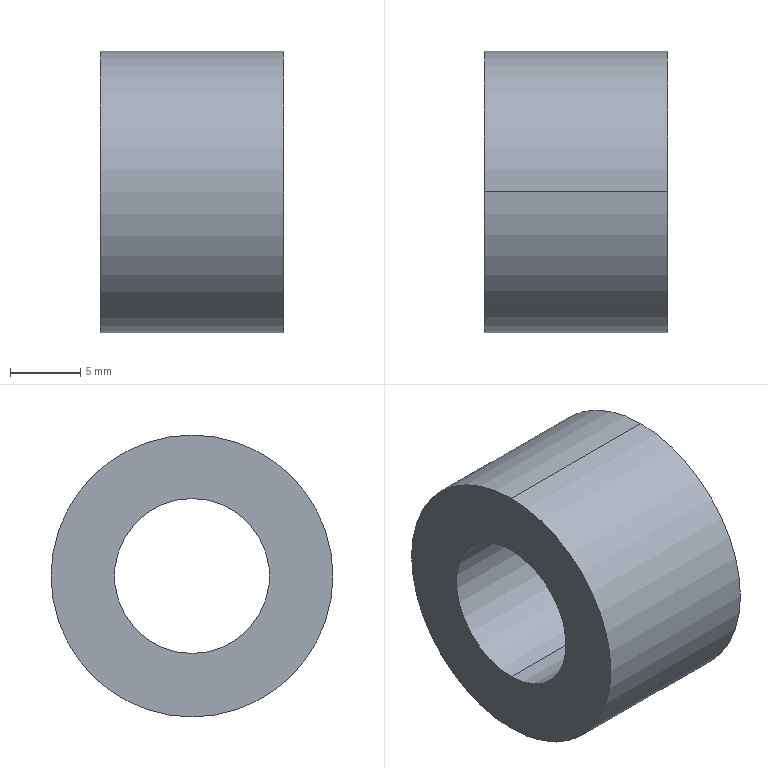Part | SolidWorks | features Extrusion 1 | 1 solid | 6 faces | box 13 x 20 x 20 mm | volume 2849 mm3 | cylinder 4 | plane 2 | commonest cylinder face diameters 11 x2 20 x2
STEP:
#1=CARTESIAN_POINT('',(6.5,0.,5.5));
#2=VERTEX_POINT('',#1);
#3=CARTESIAN_POINT('',(6.5,0.,-5.5));
#4=VERTEX_POINT('',#3);
#5=CARTESIAN_POINT('',(6.5,0.,0.));
#6=DIRECTION('',(1.,0.,0.));
#7=DIRECTION('',(0.,0.,-1.));
#8=AXIS2_PLACEMENT_3D('',#5,#6,#7);
#9=CIRCLE('',#8,5.5);
#10=EDGE_CURVE('',#2,#4,#9,.T.);
#11=ORIENTED_EDGE('',*,*,#10,.T.);
#12=CARTESIAN_POINT('',(-6.5,0.,-5.5));
#13=VERTEX_POINT('',#12);
#14=CARTESIAN_POINT('',(6.5,0.,-5.5));
#15=DIRECTION('',(-1.,0.,0.));
#16=VECTOR('',#15,1000.);
#17=LINE('',#14,#16);
#18=EDGE_CURVE('',#4,#13,#17,.T.);
#19=ORIENTED_EDGE('',*,*,#18,.T.);
#20=CARTESIAN_POINT('',(-6.5,0.,5.5));
#21=VERTEX_POINT('',#20);
#22=CARTESIAN_POINT('',(-6.5,0.,0.));
#23=DIRECTION('',(1.,0.,0.));
#24=DIRECTION('',(0.,0.,-1.));
#25=AXIS2_PLACEMENT_3D('',#22,#23,#24);
#26=CIRCLE('',#25,5.5);
#27=EDGE_CURVE('',#21,#13,#26,.T.);
#28=ORIENTED_EDGE('',*,*,#27,.F.);
#29=CARTESIAN_POINT('',(6.5,0.,5.5));
#30=DIRECTION('',(-1.,0.,0.));
#31=VECTOR('',#30,1000.);
#32=LINE('',#29,#31);
#33=EDGE_CURVE('',#2,#21,#32,.T.);
#34=ORIENTED_EDGE('',*,*,#33,.F.);
#35=EDGE_LOOP('',(#11,#19,#28,#34));
#36=FACE_OUTER_BOUND('',#35,.T.);
#37=CARTESIAN_POINT('',(6.5,0.,0.));
#38=DIRECTION('',(-1.,0.,0.));
#39=DIRECTION('',(0.,0.,1.));
#40=AXIS2_PLACEMENT_3D('',#37,#38,#39);
#41=CYLINDRICAL_SURFACE('',#40,5.5);
#42=ADVANCED_FACE('',(#36),#41,.F.);
#43=CARTESIAN_POINT('',(6.5,0.,-10.));
#44=VERTEX_POINT('',#43);
#45=CARTESIAN_POINT('',(6.5,0.,10.));
#46=VERTEX_POINT('',#45);
#47=CARTESIAN_POINT('',(6.5,0.,0.));
#48=DIRECTION('',(1.,0.,0.));
#49=DIRECTION('',(0.,0.,-1.));
#50=AXIS2_PLACEMENT_3D('',#47,#48,#49);
#51=CIRCLE('',#50,10.);
#52=EDGE_CURVE('',#44,#46,#51,.T.);
#53=ORIENTED_EDGE('',*,*,#52,.F.);
#54=CARTESIAN_POINT('',(-6.5,0.,-10.));
#55=VERTEX_POINT('',#54);
#56=CARTESIAN_POINT('',(6.5,0.,-10.));
#57=DIRECTION('',(-1.,0.,0.));
#58=VECTOR('',#57,1000.);
#59=LINE('',#56,#58);
#60=EDGE_CURVE('',#44,#55,#59,.T.);
#61=ORIENTED_EDGE('',*,*,#60,.T.);
#62=CARTESIAN_POINT('',(-6.5,0.,10.));
#63=VERTEX_POINT('',#62);
#64=CARTESIAN_POINT('',(-6.5,0.,0.));
#65=DIRECTION('',(1.,0.,0.));
#66=DIRECTION('',(0.,0.,-1.));
#67=AXIS2_PLACEMENT_3D('',#64,#65,#66);
#68=CIRCLE('',#67,10.);
#69=EDGE_CURVE('',#55,#63,#68,.T.);
#70=ORIENTED_EDGE('',*,*,#69,.T.);
#71=CARTESIAN_POINT('',(6.5,0.,10.));
#72=DIRECTION('',(-1.,0.,0.));
#73=VECTOR('',#72,1000.);
#74=LINE('',#71,#73);
#75=EDGE_CURVE('',#46,#63,#74,.T.);
#76=ORIENTED_EDGE('',*,*,#75,.F.);
#77=EDGE_LOOP('',(#53,#61,#70,#76));
#78=FACE_OUTER_BOUND('',#77,.T.);
#79=CARTESIAN_POINT('',(6.5,0.,0.));
#80=DIRECTION('',(-1.,0.,0.));
#81=DIRECTION('',(0.,0.,1.));
#82=AXIS2_PLACEMENT_3D('',#79,#80,#81);
#83=CYLINDRICAL_SURFACE('',#82,10.);
#84=ADVANCED_FACE('',(#78),#83,.T.);
#85=CARTESIAN_POINT('',(6.5,0.,0.));
#86=DIRECTION('',(1.,0.,0.));
#87=DIRECTION('',(0.,0.,-1.));
#88=AXIS2_PLACEMENT_3D('',#85,#86,#87);
#89=CIRCLE('',#88,10.);
#90=EDGE_CURVE('',#46,#44,#89,.T.);
#91=ORIENTED_EDGE('',*,*,#90,.T.);
#92=ORIENTED_EDGE('',*,*,#52,.T.);
#93=EDGE_LOOP('',(#91,#92));
#94=FACE_OUTER_BOUND('',#93,.T.);
#95=ORIENTED_EDGE('',*,*,#10,.F.);
#96=CARTESIAN_POINT('',(6.5,0.,0.));
#97=DIRECTION('',(1.,0.,0.));
#98=DIRECTION('',(0.,0.,-1.));
#99=AXIS2_PLACEMENT_3D('',#96,#97,#98);
#100=CIRCLE('',#99,5.5);
#101=EDGE_CURVE('',#4,#2,#100,.T.);
#102=ORIENTED_EDGE('',*,*,#101,.F.);
#103=EDGE_LOOP('',(#95,#102));
#104=FACE_BOUND('',#103,.T.);
#105=CARTESIAN_POINT('',(6.5,0.,0.));
#106=DIRECTION('',(1.,0.,0.));
#107=DIRECTION('',(0.,0.,-1.));
#108=AXIS2_PLACEMENT_3D('',#105,#106,#107);
#109=PLANE('',#108);
#110=ADVANCED_FACE('',(#94,#104),#109,.T.);
#111=CARTESIAN_POINT('',(-6.5,0.,0.));
#112=DIRECTION('',(1.,0.,0.));
#113=DIRECTION('',(0.,0.,-1.));
#114=AXIS2_PLACEMENT_3D('',#111,#112,#113);
#115=CIRCLE('',#114,10.);
#116=EDGE_CURVE('',#63,#55,#115,.T.);
#117=ORIENTED_EDGE('',*,*,#116,.F.);
#118=ORIENTED_EDGE('',*,*,#69,.F.);
#119=EDGE_LOOP('',(#117,#118));
#120=FACE_OUTER_BOUND('',#119,.T.);
#121=ORIENTED_EDGE('',*,*,#27,.T.);
#122=CARTESIAN_POINT('',(-6.5,0.,0.));
#123=DIRECTION('',(1.,0.,0.));
#124=DIRECTION('',(0.,0.,-1.));
#125=AXIS2_PLACEMENT_3D('',#122,#123,#124);
#126=CIRCLE('',#125,5.5);
#127=EDGE_CURVE('',#13,#21,#126,.T.);
#128=ORIENTED_EDGE('',*,*,#127,.T.);
#129=EDGE_LOOP('',(#121,#128));
#130=FACE_BOUND('',#129,.T.);
#131=CARTESIAN_POINT('',(-6.5,0.,0.));
#132=DIRECTION('',(1.,0.,0.));
#133=DIRECTION('',(0.,0.,-1.));
#134=AXIS2_PLACEMENT_3D('',#131,#132,#133);
#135=PLANE('',#134);
#136=ADVANCED_FACE('',(#120,#130),#135,.F.);
#137=ORIENTED_EDGE('',*,*,#60,.F.);
#138=ORIENTED_EDGE('',*,*,#90,.F.);
#139=ORIENTED_EDGE('',*,*,#75,.T.);
#140=ORIENTED_EDGE('',*,*,#116,.T.);
#141=EDGE_LOOP('',(#137,#138,#139,#140));
#142=FACE_OUTER_BOUND('',#141,.T.);
#143=CARTESIAN_POINT('',(6.5,0.,0.));
#144=DIRECTION('',(-1.,0.,0.));
#145=DIRECTION('',(0.,0.,1.));
#146=AXIS2_PLACEMENT_3D('',#143,#144,#145);
#147=CYLINDRICAL_SURFACE('',#146,10.);
#148=ADVANCED_FACE('',(#142),#147,.T.);
#149=ORIENTED_EDGE('',*,*,#18,.F.);
#150=ORIENTED_EDGE('',*,*,#101,.T.);
#151=ORIENTED_EDGE('',*,*,#33,.T.);
#152=ORIENTED_EDGE('',*,*,#127,.F.);
#153=EDGE_LOOP('',(#149,#150,#151,#152));
#154=FACE_OUTER_BOUND('',#153,.T.);
#155=CARTESIAN_POINT('',(6.5,0.,0.));
#156=DIRECTION('',(-1.,0.,0.));
#157=DIRECTION('',(0.,0.,1.));
#158=AXIS2_PLACEMENT_3D('',#155,#156,#157);
#159=CYLINDRICAL_SURFACE('',#158,5.5);
#160=ADVANCED_FACE('',(#154),#159,.F.);
#161=CLOSED_SHELL('',(#42,#84,#110,#136,#148,#160));
#162=MANIFOLD_SOLID_BREP('',#161);
#163=CARTESIAN_POINT('',(0.,0.,0.));
#164=DIRECTION('',(0.,0.,1.));
#165=DIRECTION('',(1.,0.,0.));
#166=AXIS2_PLACEMENT_3D('',#163,#164,#165);
#167=(LENGTH_UNIT()NAMED_UNIT(*)SI_UNIT(.MILLI.,.METRE.));
#168=UNCERTAINTY_MEASURE_WITH_UNIT(LENGTH_MEASURE(0.00001),#167,'','');
#169=(NAMED_UNIT(*)PLANE_ANGLE_UNIT()SI_UNIT($,.RADIAN.));
#170=(NAMED_UNIT(*)SI_UNIT($,.STERADIAN.)SOLID_ANGLE_UNIT());
#171=(GEOMETRIC_REPRESENTATION_CONTEXT(3)GLOBAL_UNCERTAINTY_ASSIGNED_CONTEXT((#168))GLOBAL_UNIT_ASSIGNED_CONTEXT((#167,#169,#170))REPRESENTATION_CONTEXT('',''));
#172=ADVANCED_BREP_SHAPE_REPRESENTATION('',(#162,#166),#171);